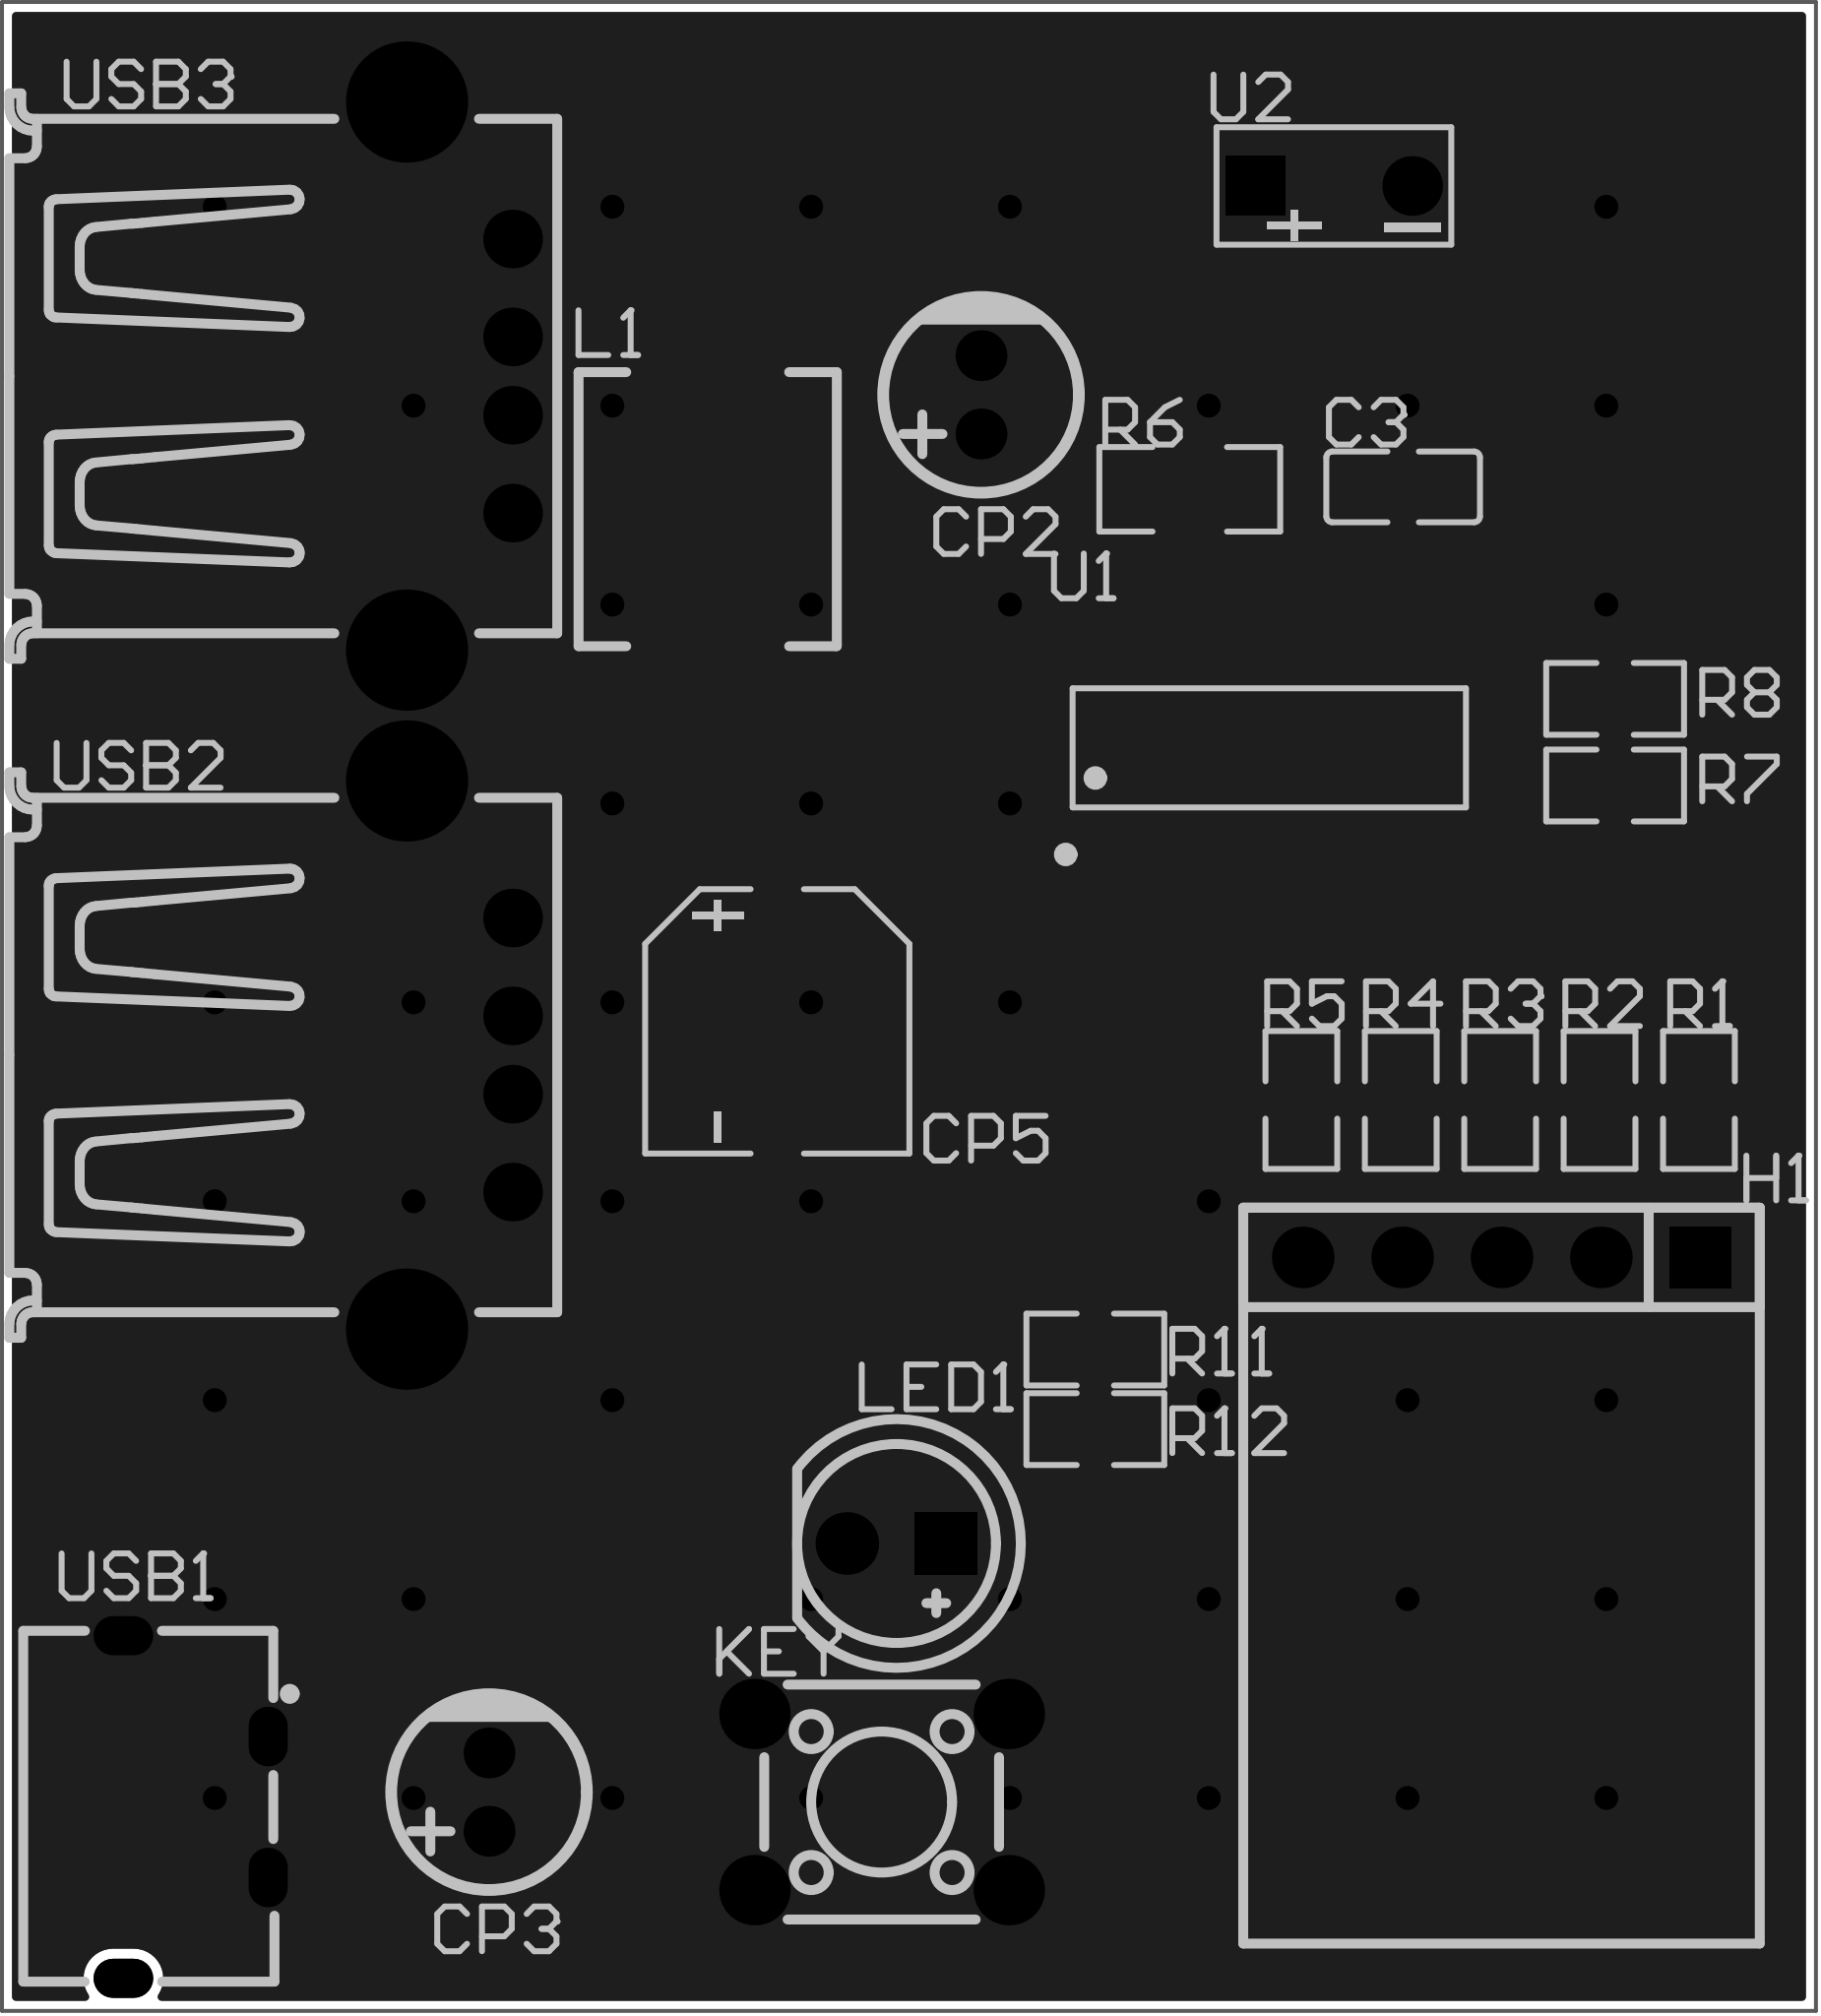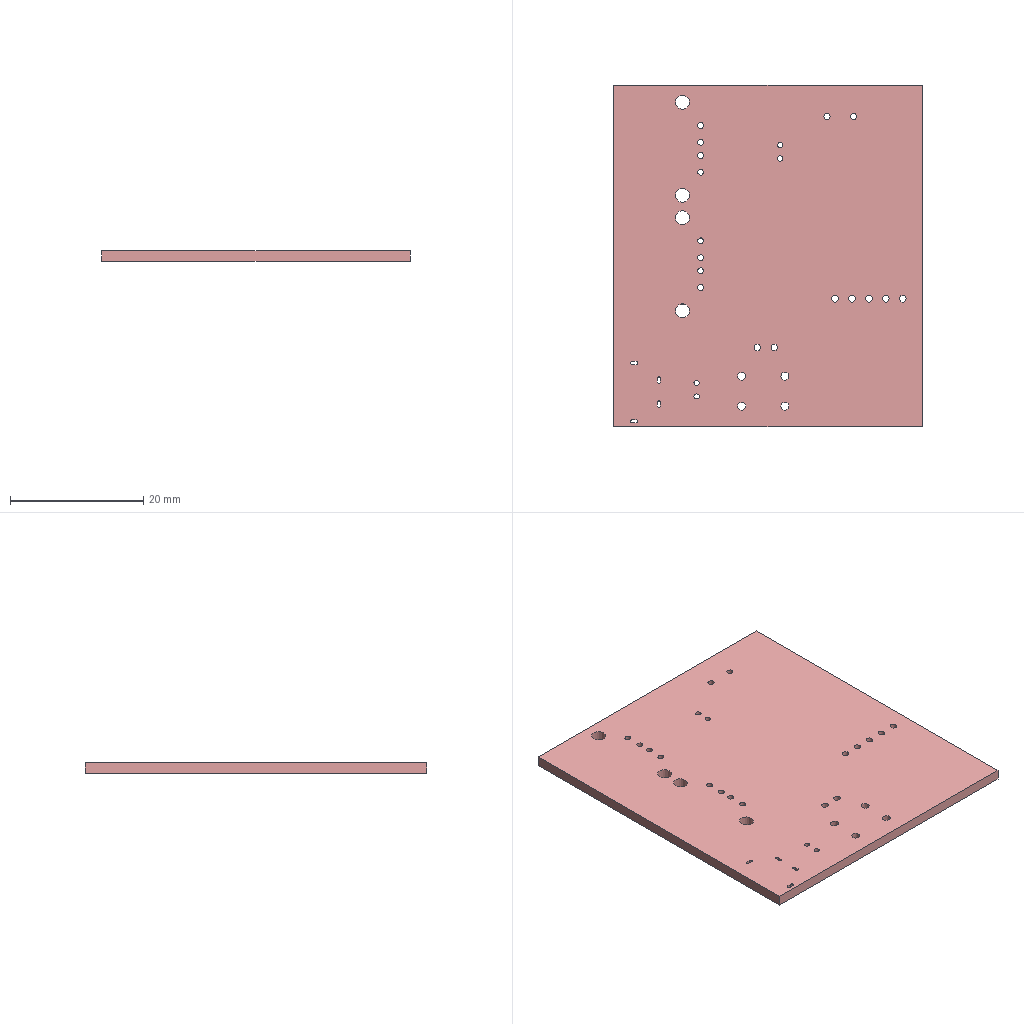Circuit board layout | Altium Designer | box 46.4 x 51.3 x 1.6 mm
Layer stack:
# Altium Designer layer stack of  (unit mm; dielectric type: 0 none, 1 core, 2 prepreg, 3 surface material)
index,name,kind,layer,copper_thickness_mm,dielectric_type,dielectric_thickness_mm,dielectric_material,dielectric_constant
0,Top Paste Mask Layer,other,,,,,,
1,Top Silkscreen Layer,other,,,,,,
2,Top Solder Mask Layer,dielectric,,,3,0.01,,3.3
3,Top Layer,copper,Top Layer,0.035,,,,
4,Dielectric1,dielectric,,,3,1.51,FR4,4.5
5,Bottom Layer,copper,Bottom Layer,0.035,,,,
6,Bottom Solder Mask Layer,dielectric,,,3,0.01,,3.3
7,Bottom Silkscreen Layer,other,,,,,,
8,Bottom Paste Mask Layer,other,,,,,,
# drill layer pairs: low layer,high layer
drill_pair,Top Layer,Bottom Layer
Part placement:
Designator,Comment,Layer,Footprint,Center-X(mm),Center-Y(mm),Rotation
C3,2.2uF,TopLayer,C0805,115.816,117.537,180
CP2,RT1_10uF/50V,TopLayer,CAP-TH_BD5.0-P2.00-D0.8-FD,105.029,119.888,90
CP3,RT1_10uF/50V,TopLayer,CAP-TH_BD5.0-P2.00-D0.8-FD,92.456,84.201,90
CP5,47uF/50V,TopLayer,CAP-SMD_BD6.3-L6.6-W6.6-LS7.0-FD,99.822,103.886,270
H1,,TopLayer,HDR-TH_5P-P2.54-V-F,118.329,97.858,180
KEY,,TopLayer,SW-TH_4P-L6.0-W6.0-P4.50-LS6.5,102.489,83.947,0
L1,1uH,TopLayer,IND-SMD_L7.0-W6.6,98.044,116.967,270
LED1,,TopLayer,LED-TH_5mm,102.87,90.551,180
R1,510R,TopLayer,R0805,123.375,101.878,270
R2,510R,TopLayer,R0805,120.835,101.878,270
R3,510R,TopLayer,R0805,118.295,101.878,270
R4,510R,TopLayer,R0805,115.755,101.878,270
R5,510R,TopLayer,R0805,113.215,101.878,270
R6,合金电阻,0.01R,TopLayer,R1206,110.363,117.475,180
R7,15K,TopLayer,R0805,121.233,109.91,0
R8,1K,TopLayer,R0805,121.233,112.122,0
R11,10K,TopLayer,R0805,107.95,95.504,180
R12,20R,TopLayer,R0805,107.95,93.472,180
U1,IP5506-BZ-188,TopLayer,ESOP-16_L9.9-W3.9-P1.27-LS6.0-BL-EP,112.395,110.871,0
U2,电池盒接口,TopLayer,TH_C9900019910,114.046,125.222,0
USB1,KH-TYPE-C-2P,TopLayer,USB-SMD_KH-TYPE-C-2P,84.963,83.82,270
USB2,,TopLayer,USB__Type-A,91.704,103.026,270
USB3,,TopLayer,USB__Type-A,91.704,120.367,270
Pad and via stacks:
# Altium Designer via and pad stacks of  (unit mm). Each distinct definition once, with the count of objects using it.
# via: kind,start_layer,end_layer,hole_mm,diameter_mm,mode(0 simple;1 top-mid-bottom;2 full stack),diameter_per_layer,count,example_net
# pad: kind,layer,hole_mm,hole_type(0 round;1 square;2 slot),plating,top_size,top_shape(1 round;2 rect;3 octagon;9 rounded rect),mid_size,bottom_size,mode,footprint,size_per_layer,count,example
pad,Top Layer,0,0,plated,1.41x1.35,2,1.41x1.35,1.41x1.35,0,C0805,,2,C3.2
pad,Top Layer,0,0,plated,3.06x1,2,3.06x1,3.06x1,0,CAP-SMD_BD6.3-L6.6-W6.6-LS7.0-FD,,2,CP5.1
pad,Top Layer,0,0,plated,2.4x3.2,2,2.4x3.2,2.4x3.2,0,IND-SMD_L7.0-W6.6,,2,L1.1
pad,Top Layer,0,0,plated,1.133x1.377,2,1.133x1.377,1.133x1.377,0,R0805,,18,R1.2
pad,Top Layer,0,0,plated,1.208x1.701,2,1.208x1.701,1.208x1.701,0,R1206,,2,R6.2
pad,Top Layer,0,0,plated,0.609x1.944,1,0.609x1.944,0.609x1.944,0,ESOP-16_L9.9-W3.9-P1.27-LS6.0-BL-EP,,16,U1.1
pad,Top Layer,0,0,plated,4.57x2.41,2,4.57x2.41,4.57x2.41,0,ESOP-16_L9.9-W3.9-P1.27-LS6.0-BL-EP,,1,U1.17
pad,Multi-Layer,0.8,0,plated,1.3x1.3,1,1.3x1.3,1.3x1.3,0,CAP-TH_BD5.0-P2.00-D0.8-FD,,4,CP2.1
pad,Multi-Layer,1.02,0,plated,1.575x1.575,1,1.575x1.575,1.575x1.575,0,HDR-TH_5P-P2.54-V-F,,4,H1.5
pad,Multi-Layer,1.02,0,plated,1.575x1.575,2,1.575x1.575,1.575x1.575,0,HDR-TH_5P-P2.54-V-F,,1,H1.1
pad,Multi-Layer,1.2,0,plated,1.8x1.8,1,1.8x1.8,1.8x1.8,0,SW-TH_4P-L6.0-W6.0-P4.50-LS6.5,,4,KEY.1
pad,Multi-Layer,1,0,plated,1.6x1.6,2,1.6x1.6,1.6x1.6,0,LED-TH_5mm,,1,LED1.1
pad,Multi-Layer,1,0,plated,1.6x1.6,1,1.6x1.6,1.6x1.6,0,LED-TH_5mm,,1,LED1.2
pad,Multi-Layer,0.9144,0,plated,1.524x1.524,2,1.524x1.524,1.524x1.524,0,TH_C9900019910,,1,U2.1
pad,Multi-Layer,0.9144,0,plated,1.524x1.524,1,1.524x1.524,1.524x1.524,0,TH_C9900019910,,1,U2.2
pad,Multi-Layer,0.45,2,plated,1x1.524,1,1x1.524,1x1.524,0,USB-SMD_KH-TYPE-C-2P,,2,USB1.1
pad,Multi-Layer,0.5,2,plated,1x1.524,1,1x1.524,1x1.524,0,USB-SMD_KH-TYPE-C-2P,,2,USB1.3
pad,Multi-Layer,2.1,0,plated,3.1x3.1,1,3.1x3.1,3.1x3.1,0,USB_ Type-A,,4,USB2.SH2
pad,Multi-Layer,0.9,0,plated,1.5x1.5,1,1.5x1.5,1.5x1.5,0,USB_ Type-A,,8,USB2.1
via,Top Layer,Bottom Layer,0.3048,0.61,0,,47,GND
Copper pours:
name,layer,net,type(0 solid;1 hatched;2 none)
Top Layer-GND,Top Layer,GND,0
Bottom Layer-GND,Bottom Layer,GND,0